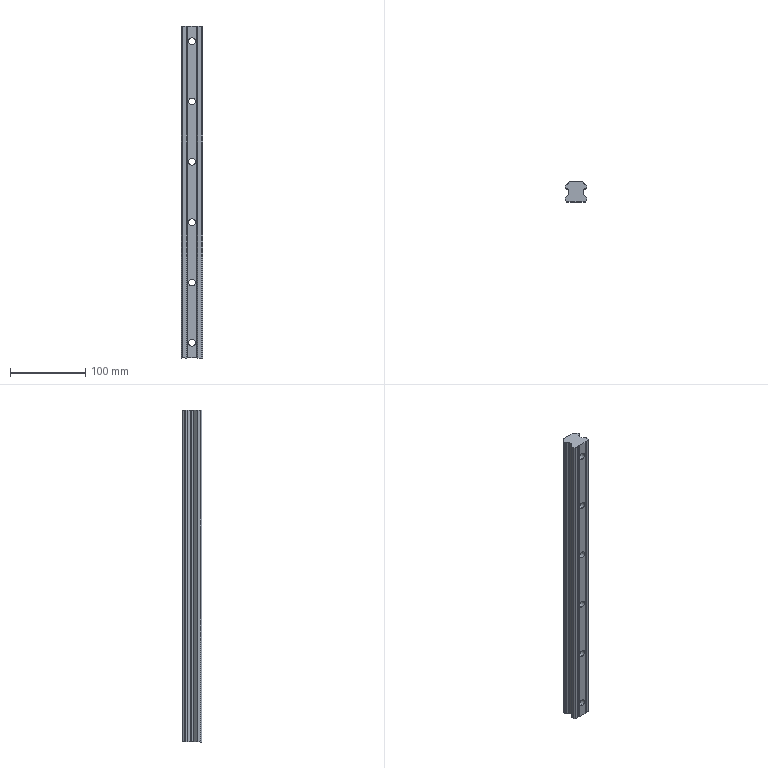Part | SolidWorks | features BaseBody 1 | 1 solid | 82 faces | box 28 x 26 x 440 mm | volume 253404 mm3 | cylinder 46 | plane 36 | commonest cylinder face diameters 1.2 x12 9 x12 14 x12 1.6 x6 5.66 x4